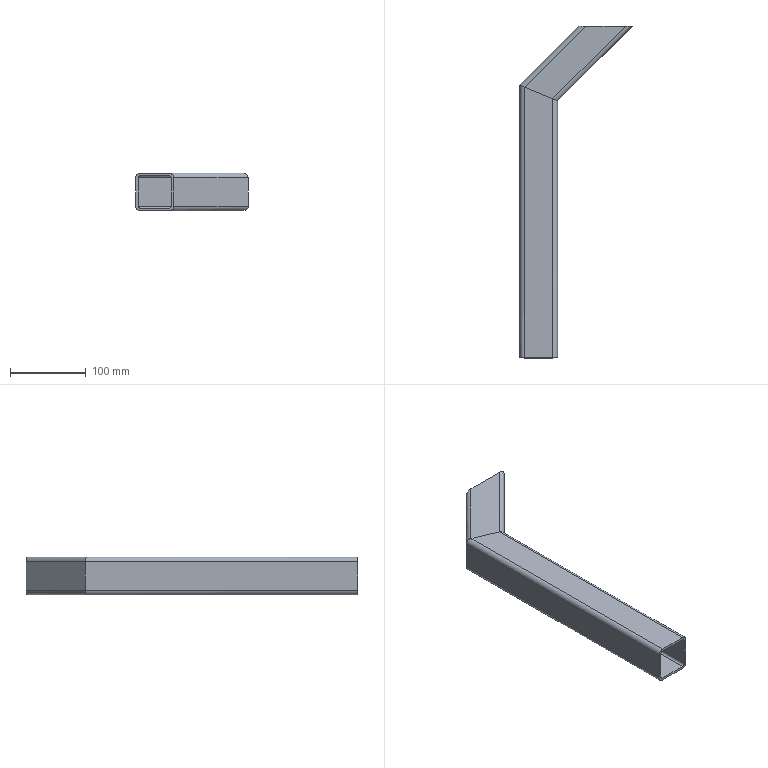Part | STEP file | Column square tube SGN-7-02_Default<machined> | 2 solids | 36 faces | box 148.744 x 438.388 x 50 mm | volume 272018 mm3 | plane 20 | cylinder 16 | commonest cylinder face diameters 6.4 x8 12.8 x8